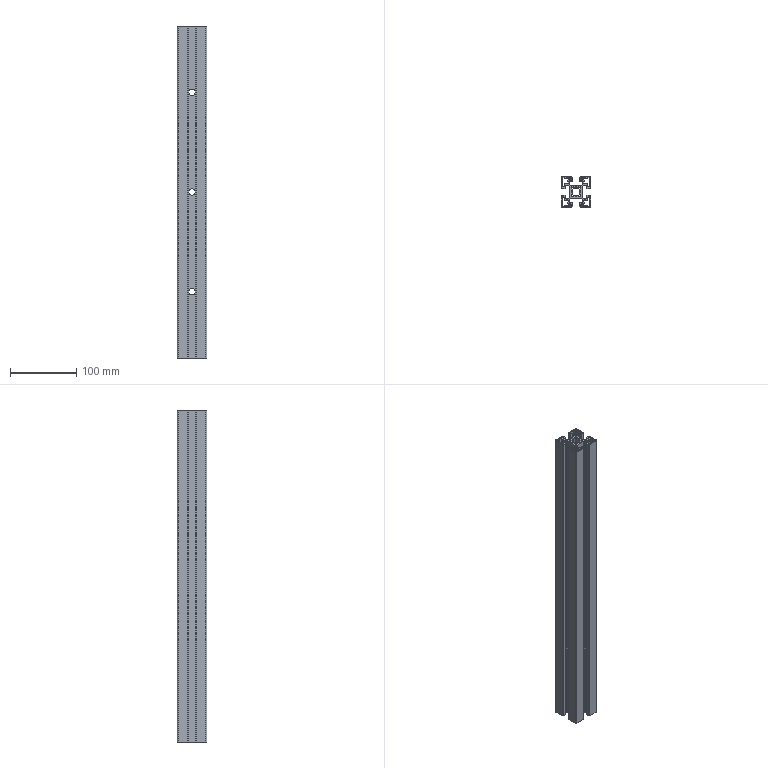Part | SolidWorks | features Extrusion 1, HoleWzd 1 | 1 solid | 326 faces | box 45 x 45 x 500 mm | volume 317021 mm3 | plane 238 | cylinder 88 | commonest cylinder face diameters 2 x36 12 x20 10 x12 3 x10 15 x6 4 x4